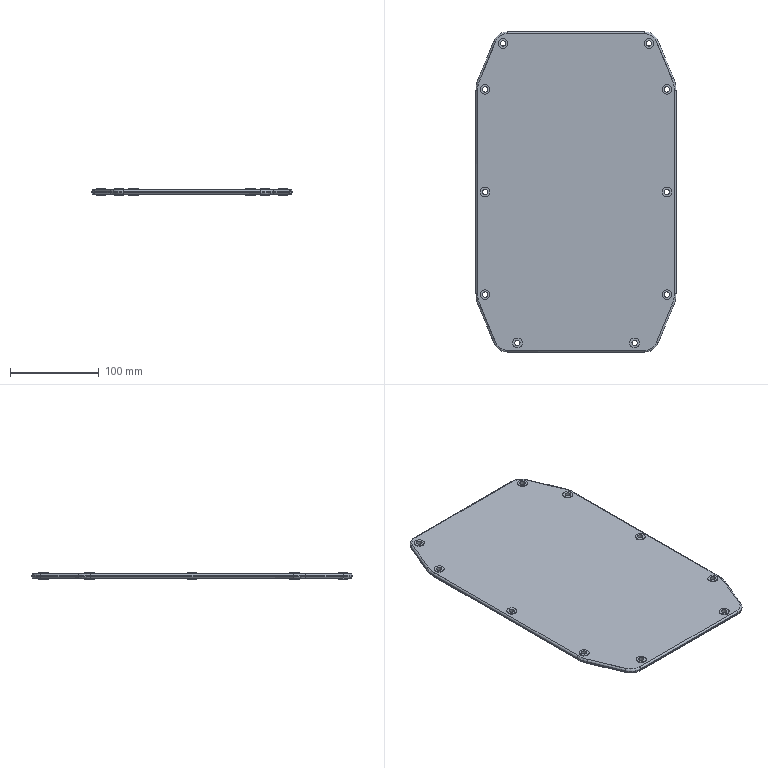Part | SolidWorks | features BaseBody 1 | 1 solid | 229 faces | box 225 x 360 x 7 mm | volume 388175 mm3 | cylinder 183 | plane 30 | torus 16 | commonest cylinder face diameters 11.001 x80 6 x59 4 x32 31.931 x8 71.945 x1 71.953 x1